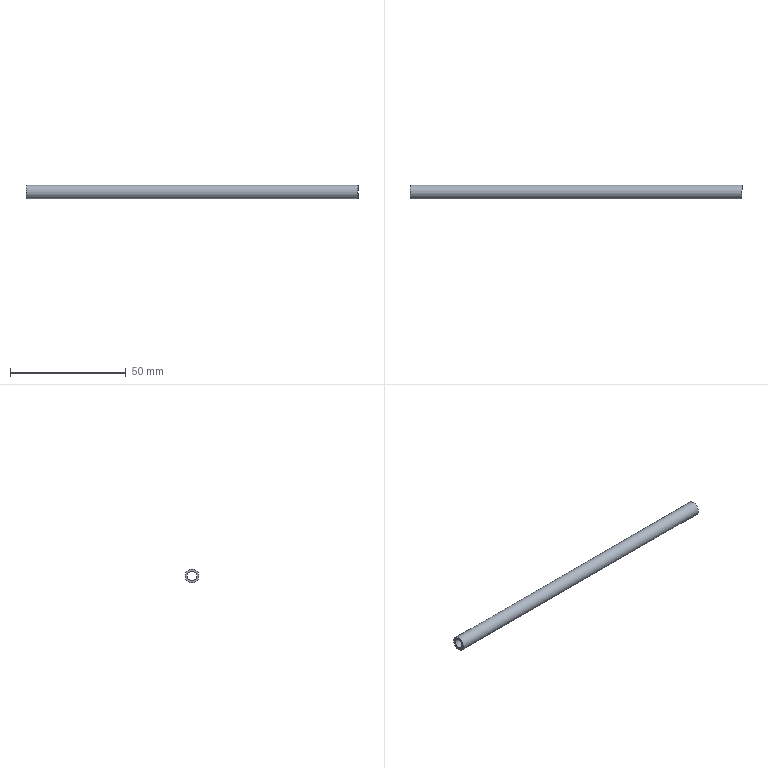Part | NX | features solid 2 | 1 solid | 4 faces | box 143.315 x 6 x 6 mm | volume 2251 mm3 | cylinder 2 | plane 2 | commonest cylinder face diameters 4 x1 6 x1
STEP:
#1=CARTESIAN_POINT('',(-153.315,47.,347.));
#2=VERTEX_POINT('',#1);
#3=CARTESIAN_POINT('',(-153.315,45.,347.));
#4=DIRECTION('',(1.,0.,0.));
#5=DIRECTION('',(0.,1.,0.));
#6=AXIS2_PLACEMENT_3D('',#3,#4,#5);
#7=CIRCLE('',#6,2.);
#8=EDGE_CURVE('',#2,#2,#7,.F.);
#9=ORIENTED_EDGE('',*,*,#8,.T.);
#10=EDGE_LOOP('',(#9));
#11=FACE_BOUND('',#10,.T.);
#12=CARTESIAN_POINT('',(-10.,43.,347.));
#13=VERTEX_POINT('',#12);
#14=CARTESIAN_POINT('',(-10.,45.,347.));
#15=DIRECTION('',(-1.,0.,0.));
#16=DIRECTION('',(0.,-1.,0.));
#17=AXIS2_PLACEMENT_3D('',#14,#15,#16);
#18=CIRCLE('',#17,2.);
#19=EDGE_CURVE('',#13,#13,#18,.T.);
#20=ORIENTED_EDGE('',*,*,#19,.F.);
#21=EDGE_LOOP('',(#20));
#22=FACE_BOUND('',#21,.T.);
#23=CARTESIAN_POINT('',(-288.824,45.,347.));
#24=DIRECTION('',(1.,0.,0.));
#25=DIRECTION('',(0.,1.,0.));
#26=AXIS2_PLACEMENT_3D('',#23,#24,#25);
#27=CYLINDRICAL_SURFACE('',#26,2.);
#28=ADVANCED_FACE('',(#11,#22),#27,.F.);
#29=CARTESIAN_POINT('',(-153.315,48.,347.));
#30=VERTEX_POINT('',#29);
#31=CARTESIAN_POINT('',(-153.315,45.,347.));
#32=DIRECTION('',(1.,0.,0.));
#33=DIRECTION('',(0.,1.,0.));
#34=AXIS2_PLACEMENT_3D('',#31,#32,#33);
#35=CIRCLE('',#34,3.);
#36=EDGE_CURVE('',#30,#30,#35,.F.);
#37=ORIENTED_EDGE('',*,*,#36,.F.);
#38=EDGE_LOOP('',(#37));
#39=FACE_BOUND('',#38,.T.);
#40=CARTESIAN_POINT('',(-10.,42.,347.));
#41=VERTEX_POINT('',#40);
#42=CARTESIAN_POINT('',(-10.,45.,347.));
#43=DIRECTION('',(-1.,0.,0.));
#44=DIRECTION('',(0.,-1.,0.));
#45=AXIS2_PLACEMENT_3D('',#42,#43,#44);
#46=CIRCLE('',#45,3.);
#47=EDGE_CURVE('',#41,#41,#46,.T.);
#48=ORIENTED_EDGE('',*,*,#47,.T.);
#49=EDGE_LOOP('',(#48));
#50=FACE_BOUND('',#49,.T.);
#51=CARTESIAN_POINT('',(-288.824,45.,347.));
#52=DIRECTION('',(1.,0.,0.));
#53=DIRECTION('',(0.,1.,0.));
#54=AXIS2_PLACEMENT_3D('',#51,#52,#53);
#55=CYLINDRICAL_SURFACE('',#54,3.);
#56=ADVANCED_FACE('',(#39,#50),#55,.T.);
#57=ORIENTED_EDGE('',*,*,#8,.F.);
#58=EDGE_LOOP('',(#57));
#59=FACE_BOUND('',#58,.T.);
#60=ORIENTED_EDGE('',*,*,#36,.T.);
#61=EDGE_LOOP('',(#60));
#62=FACE_BOUND('',#61,.T.);
#63=CARTESIAN_POINT('',(-153.315,28.272,168.));
#64=DIRECTION('',(1.,0.,0.));
#65=DIRECTION('',(0.,1.,0.));
#66=AXIS2_PLACEMENT_3D('',#63,#64,#65);
#67=PLANE('',#66);
#68=ADVANCED_FACE('',(#59,#62),#67,.F.);
#69=ORIENTED_EDGE('',*,*,#19,.T.);
#70=EDGE_LOOP('',(#69));
#71=FACE_BOUND('',#70,.T.);
#72=ORIENTED_EDGE('',*,*,#47,.F.);
#73=EDGE_LOOP('',(#72));
#74=FACE_BOUND('',#73,.T.);
#75=CARTESIAN_POINT('',(-10.,45.,347.));
#76=DIRECTION('',(-1.,0.,0.));
#77=DIRECTION('',(0.,-1.,0.));
#78=AXIS2_PLACEMENT_3D('',#75,#76,#77);
#79=PLANE('',#78);
#80=ADVANCED_FACE('',(#71,#74),#79,.F.);
#81=CLOSED_SHELL('',(#28,#56,#68,#80));
#82=MANIFOLD_SOLID_BREP('',#81);
#83=(LENGTH_UNIT()NAMED_UNIT(*)SI_UNIT(.MILLI.,.METRE.));
#84=UNCERTAINTY_MEASURE_WITH_UNIT(LENGTH_MEASURE(0.00001),#83,'','');
#85=(NAMED_UNIT(*)PLANE_ANGLE_UNIT()SI_UNIT($,.RADIAN.));
#86=(NAMED_UNIT(*)SI_UNIT($,.STERADIAN.)SOLID_ANGLE_UNIT());
#87=(GEOMETRIC_REPRESENTATION_CONTEXT(3)GLOBAL_UNCERTAINTY_ASSIGNED_CONTEXT((#84))GLOBAL_UNIT_ASSIGNED_CONTEXT((#83,#85,#86))REPRESENTATION_CONTEXT('',''));
#88=ADVANCED_BREP_SHAPE_REPRESENTATION('',(#82),#87);